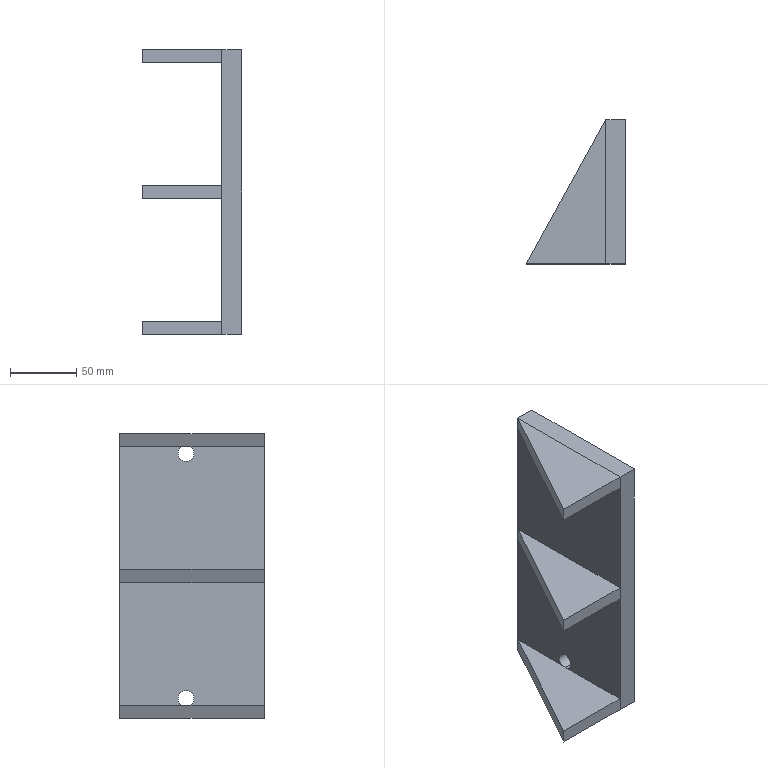Part | SolidWorks | features Extrusion 1, HoleWzd 1, ICE 1, LPattern 1, WeldmentFeature 1 | 4 solids | 30 faces | box 75 x 109 x 215 mm | volume 446232 mm3 | plane 23 | cylinder 7 | commonest cylinder face diameters 12 x7
STEP:
#1=CARTESIAN_POINT('',(-15.,0.,112.5));
#2=VERTEX_POINT('',#1);
#3=CARTESIAN_POINT('',(-15.,109.,112.5));
#4=VERTEX_POINT('',#3);
#5=CARTESIAN_POINT('',(-15.,0.,112.5));
#6=DIRECTION('',(0.,1.,0.));
#7=VECTOR('',#6,1000.);
#8=LINE('',#5,#7);
#9=EDGE_CURVE('',#2,#4,#8,.T.);
#10=ORIENTED_EDGE('',*,*,#9,.F.);
#11=CARTESIAN_POINT('',(-15.,0.,102.5));
#12=VERTEX_POINT('',#11);
#13=CARTESIAN_POINT('',(-15.,0.,102.5));
#14=DIRECTION('',(0.,0.,1.));
#15=VECTOR('',#14,1000.);
#16=LINE('',#13,#15);
#17=EDGE_CURVE('',#12,#2,#16,.T.);
#18=ORIENTED_EDGE('',*,*,#17,.F.);
#19=CARTESIAN_POINT('',(-15.,109.,102.5));
#20=VERTEX_POINT('',#19);
#21=CARTESIAN_POINT('',(-15.,0.,102.5));
#22=DIRECTION('',(0.,1.,0.));
#23=VECTOR('',#22,1000.);
#24=LINE('',#21,#23);
#25=EDGE_CURVE('',#12,#20,#24,.T.);
#26=ORIENTED_EDGE('',*,*,#25,.T.);
#27=CARTESIAN_POINT('',(-15.,109.,102.5));
#28=DIRECTION('',(0.,0.,1.));
#29=VECTOR('',#28,1000.);
#30=LINE('',#27,#29);
#31=EDGE_CURVE('',#20,#4,#30,.T.);
#32=ORIENTED_EDGE('',*,*,#31,.T.);
#33=EDGE_LOOP('',(#10,#18,#26,#32));
#34=FACE_OUTER_BOUND('',#33,.T.);
#35=CARTESIAN_POINT('',(-15.,0.,102.5));
#36=DIRECTION('',(1.,0.,0.));
#37=DIRECTION('',(0.,1.,0.));
#38=AXIS2_PLACEMENT_3D('',#35,#36,#37);
#39=PLANE('',#38);
#40=ADVANCED_FACE('',(#34),#39,.T.);
#41=CARTESIAN_POINT('',(-75.,0.,112.5));
#42=VERTEX_POINT('',#41);
#43=CARTESIAN_POINT('',(-75.,0.,112.5));
#44=DIRECTION('',(1.,0.,0.));
#45=VECTOR('',#44,1000.);
#46=LINE('',#43,#45);
#47=EDGE_CURVE('',#42,#2,#46,.T.);
#48=ORIENTED_EDGE('',*,*,#47,.F.);
#49=CARTESIAN_POINT('',(-75.,0.,102.5));
#50=VERTEX_POINT('',#49);
#51=CARTESIAN_POINT('',(-75.,0.,102.5));
#52=DIRECTION('',(0.,0.,1.));
#53=VECTOR('',#52,1000.);
#54=LINE('',#51,#53);
#55=EDGE_CURVE('',#50,#42,#54,.T.);
#56=ORIENTED_EDGE('',*,*,#55,.F.);
#57=CARTESIAN_POINT('',(-75.,0.,102.5));
#58=DIRECTION('',(1.,0.,0.));
#59=VECTOR('',#58,1000.);
#60=LINE('',#57,#59);
#61=EDGE_CURVE('',#50,#12,#60,.T.);
#62=ORIENTED_EDGE('',*,*,#61,.T.);
#63=ORIENTED_EDGE('',*,*,#17,.T.);
#64=EDGE_LOOP('',(#48,#56,#62,#63));
#65=FACE_OUTER_BOUND('',#64,.T.);
#66=CARTESIAN_POINT('',(-75.,0.,102.5));
#67=DIRECTION('',(0.,-1.,0.));
#68=DIRECTION('',(1.,0.,0.));
#69=AXIS2_PLACEMENT_3D('',#66,#67,#68);
#70=PLANE('',#69);
#71=ADVANCED_FACE('',(#65),#70,.T.);
#72=CARTESIAN_POINT('',(-15.,109.,112.5));
#73=DIRECTION('',(-0.4822,-0.876,0.));
#74=VECTOR('',#73,1000.);
#75=LINE('',#72,#74);
#76=EDGE_CURVE('',#4,#42,#75,.T.);
#77=ORIENTED_EDGE('',*,*,#76,.F.);
#78=ORIENTED_EDGE('',*,*,#31,.F.);
#79=CARTESIAN_POINT('',(-15.,109.,102.5));
#80=DIRECTION('',(-0.4822,-0.876,0.));
#81=VECTOR('',#80,1000.);
#82=LINE('',#79,#81);
#83=EDGE_CURVE('',#20,#50,#82,.T.);
#84=ORIENTED_EDGE('',*,*,#83,.T.);
#85=ORIENTED_EDGE('',*,*,#55,.T.);
#86=EDGE_LOOP('',(#77,#78,#84,#85));
#87=FACE_OUTER_BOUND('',#86,.T.);
#88=CARTESIAN_POINT('',(-15.,109.,102.5));
#89=DIRECTION('',(-0.876,0.4822,0.));
#90=DIRECTION('',(-0.4822,-0.876,0.));
#91=AXIS2_PLACEMENT_3D('',#88,#89,#90);
#92=PLANE('',#91);
#93=ADVANCED_FACE('',(#87),#92,.T.);
#94=ORIENTED_EDGE('',*,*,#25,.F.);
#95=ORIENTED_EDGE('',*,*,#61,.F.);
#96=ORIENTED_EDGE('',*,*,#83,.F.);
#97=EDGE_LOOP('',(#94,#95,#96));
#98=FACE_OUTER_BOUND('',#97,.T.);
#99=CARTESIAN_POINT('',(0.,0.,102.5));
#100=DIRECTION('',(0.,0.,-1.));
#101=DIRECTION('',(-1.,0.,0.));
#102=AXIS2_PLACEMENT_3D('',#99,#100,#101);
#103=PLANE('',#102);
#104=ADVANCED_FACE('',(#98),#103,.T.);
#105=ORIENTED_EDGE('',*,*,#9,.T.);
#106=ORIENTED_EDGE('',*,*,#76,.T.);
#107=ORIENTED_EDGE('',*,*,#47,.T.);
#108=EDGE_LOOP('',(#105,#106,#107));
#109=FACE_OUTER_BOUND('',#108,.T.);
#110=CARTESIAN_POINT('',(0.,0.,112.5));
#111=DIRECTION('',(0.,0.,-1.));
#112=DIRECTION('',(-1.,0.,0.));
#113=AXIS2_PLACEMENT_3D('',#110,#111,#112);
#114=PLANE('',#113);
#115=ADVANCED_FACE('',(#109),#114,.F.);
#116=CLOSED_SHELL('',(#40,#71,#93,#104,#115));
#117=MANIFOLD_SOLID_BREP('',#116);
#118=CARTESIAN_POINT('',(-15.,59.,206.));
#119=VERTEX_POINT('',#118);
#120=CARTESIAN_POINT('',(-15.,59.,194.));
#121=VERTEX_POINT('',#120);
#122=CARTESIAN_POINT('',(-15.,59.,200.));
#123=DIRECTION('',(1.,0.,0.));
#124=DIRECTION('',(0.,1.,0.));
#125=AXIS2_PLACEMENT_3D('',#122,#123,#124);
#126=CIRCLE('',#125,6.);
#127=EDGE_CURVE('',#119,#121,#126,.T.);
#128=ORIENTED_EDGE('',*,*,#127,.F.);
#129=CARTESIAN_POINT('',(0.,59.,206.));
#130=VERTEX_POINT('',#129);
#131=CARTESIAN_POINT('',(0.,59.,206.));
#132=DIRECTION('',(1.,0.,0.));
#133=VECTOR('',#132,1000.);
#134=LINE('',#131,#133);
#135=EDGE_CURVE('',#119,#130,#134,.T.);
#136=ORIENTED_EDGE('',*,*,#135,.T.);
#137=CARTESIAN_POINT('',(0.,59.,194.));
#138=VERTEX_POINT('',#137);
#139=CARTESIAN_POINT('',(0.,59.,200.));
#140=DIRECTION('',(1.,0.,0.));
#141=DIRECTION('',(0.,0.,-1.));
#142=AXIS2_PLACEMENT_3D('',#139,#140,#141);
#143=CIRCLE('',#142,6.);
#144=EDGE_CURVE('',#130,#138,#143,.T.);
#145=ORIENTED_EDGE('',*,*,#144,.T.);
#146=CARTESIAN_POINT('',(0.,59.,194.));
#147=DIRECTION('',(1.,0.,0.));
#148=VECTOR('',#147,1000.);
#149=LINE('',#146,#148);
#150=EDGE_CURVE('',#121,#138,#149,.T.);
#151=ORIENTED_EDGE('',*,*,#150,.F.);
#152=EDGE_LOOP('',(#128,#136,#145,#151));
#153=FACE_OUTER_BOUND('',#152,.T.);
#154=CARTESIAN_POINT('',(0.,59.,200.));
#155=DIRECTION('',(1.,0.,0.));
#156=DIRECTION('',(0.,0.,-1.));
#157=AXIS2_PLACEMENT_3D('',#154,#155,#156);
#158=CYLINDRICAL_SURFACE('',#157,6.);
#159=ADVANCED_FACE('',(#153),#158,.F.);
#160=CARTESIAN_POINT('',(-15.,59.,21.));
#161=VERTEX_POINT('',#160);
#162=CARTESIAN_POINT('',(-15.,59.,9.));
#163=VERTEX_POINT('',#162);
#164=CARTESIAN_POINT('',(-15.,59.,15.));
#165=DIRECTION('',(1.,0.,0.));
#166=DIRECTION('',(0.,1.,0.));
#167=AXIS2_PLACEMENT_3D('',#164,#165,#166);
#168=CIRCLE('',#167,6.);
#169=EDGE_CURVE('',#161,#163,#168,.T.);
#170=ORIENTED_EDGE('',*,*,#169,.F.);
#171=CARTESIAN_POINT('',(0.,59.,21.));
#172=VERTEX_POINT('',#171);
#173=CARTESIAN_POINT('',(0.,59.,21.));
#174=DIRECTION('',(1.,0.,0.));
#175=VECTOR('',#174,1000.);
#176=LINE('',#173,#175);
#177=EDGE_CURVE('',#161,#172,#176,.T.);
#178=ORIENTED_EDGE('',*,*,#177,.T.);
#179=CARTESIAN_POINT('',(0.,59.,9.));
#180=VERTEX_POINT('',#179);
#181=CARTESIAN_POINT('',(0.,59.,15.));
#182=DIRECTION('',(1.,0.,0.));
#183=DIRECTION('',(0.,0.,-1.));
#184=AXIS2_PLACEMENT_3D('',#181,#182,#183);
#185=CIRCLE('',#184,6.);
#186=EDGE_CURVE('',#172,#180,#185,.T.);
#187=ORIENTED_EDGE('',*,*,#186,.T.);
#188=CARTESIAN_POINT('',(0.,59.,9.));
#189=DIRECTION('',(1.,0.,0.));
#190=VECTOR('',#189,1000.);
#191=LINE('',#188,#190);
#192=EDGE_CURVE('',#163,#180,#191,.T.);
#193=ORIENTED_EDGE('',*,*,#192,.F.);
#194=EDGE_LOOP('',(#170,#178,#187,#193));
#195=FACE_OUTER_BOUND('',#194,.T.);
#196=CARTESIAN_POINT('',(0.,59.,15.));
#197=DIRECTION('',(1.,0.,0.));
#198=DIRECTION('',(0.,0.,-1.));
#199=AXIS2_PLACEMENT_3D('',#196,#197,#198);
#200=CYLINDRICAL_SURFACE('',#199,6.);
#201=ADVANCED_FACE('',(#195),#200,.F.);
#202=CARTESIAN_POINT('',(0.,0.,0.));
#203=VERTEX_POINT('',#202);
#204=CARTESIAN_POINT('',(0.,109.,0.));
#205=VERTEX_POINT('',#204);
#206=CARTESIAN_POINT('',(0.,109.,0.));
#207=DIRECTION('',(0.,1.,0.));
#208=VECTOR('',#207,1000.);
#209=LINE('',#206,#208);
#210=EDGE_CURVE('',#203,#205,#209,.T.);
#211=ORIENTED_EDGE('',*,*,#210,.T.);
#212=CARTESIAN_POINT('',(0.,109.,215.));
#213=VERTEX_POINT('',#212);
#214=CARTESIAN_POINT('',(0.,109.,215.));
#215=DIRECTION('',(0.,0.,-1.));
#216=VECTOR('',#215,1000.);
#217=LINE('',#214,#216);
#218=EDGE_CURVE('',#213,#205,#217,.T.);
#219=ORIENTED_EDGE('',*,*,#218,.F.);
#220=CARTESIAN_POINT('',(0.,0.,215.));
#221=VERTEX_POINT('',#220);
#222=CARTESIAN_POINT('',(0.,109.,215.));
#223=DIRECTION('',(0.,1.,0.));
#224=VECTOR('',#223,1000.);
#225=LINE('',#222,#224);
#226=EDGE_CURVE('',#221,#213,#225,.T.);
#227=ORIENTED_EDGE('',*,*,#226,.F.);
#228=CARTESIAN_POINT('',(0.,0.,215.));
#229=DIRECTION('',(0.,0.,-1.));
#230=VECTOR('',#229,1000.);
#231=LINE('',#228,#230);
#232=EDGE_CURVE('',#221,#203,#231,.T.);
#233=ORIENTED_EDGE('',*,*,#232,.T.);
#234=EDGE_LOOP('',(#211,#219,#227,#233));
#235=FACE_OUTER_BOUND('',#234,.T.);
#236=CARTESIAN_POINT('',(0.,59.,15.));
#237=DIRECTION('',(1.,0.,0.));
#238=DIRECTION('',(0.,0.,-1.));
#239=AXIS2_PLACEMENT_3D('',#236,#237,#238);
#240=CIRCLE('',#239,6.);
#241=EDGE_CURVE('',#180,#172,#240,.T.);
#242=ORIENTED_EDGE('',*,*,#241,.F.);
#243=ORIENTED_EDGE('',*,*,#186,.F.);
#244=EDGE_LOOP('',(#242,#243));
#245=FACE_BOUND('',#244,.T.);
#246=CARTESIAN_POINT('',(0.,59.,200.));
#247=DIRECTION('',(1.,0.,0.));
#248=DIRECTION('',(0.,0.,-1.));
#249=AXIS2_PLACEMENT_3D('',#246,#247,#248);
#250=CIRCLE('',#249,6.);
#251=EDGE_CURVE('',#138,#130,#250,.T.);
#252=ORIENTED_EDGE('',*,*,#251,.F.);
#253=ORIENTED_EDGE('',*,*,#144,.F.);
#254=EDGE_LOOP('',(#252,#253));
#255=FACE_BOUND('',#254,.T.);
#256=CARTESIAN_POINT('',(0.,109.,215.));
#257=DIRECTION('',(-1.,0.,0.));
#258=DIRECTION('',(0.,-1.,0.));
#259=AXIS2_PLACEMENT_3D('',#256,#257,#258);
#260=PLANE('',#259);
#261=ADVANCED_FACE('',(#235,#245,#255),#260,.F.);
#262=CARTESIAN_POINT('',(-15.,109.,0.));
#263=VERTEX_POINT('',#262);
#264=CARTESIAN_POINT('',(-15.,109.,0.));
#265=DIRECTION('',(-1.,0.,0.));
#266=VECTOR('',#265,1000.);
#267=LINE('',#264,#266);
#268=EDGE_CURVE('',#205,#263,#267,.T.);
#269=ORIENTED_EDGE('',*,*,#268,.T.);
#270=CARTESIAN_POINT('',(-15.,109.,215.));
#271=VERTEX_POINT('',#270);
#272=CARTESIAN_POINT('',(-15.,109.,215.));
#273=DIRECTION('',(0.,0.,-1.));
#274=VECTOR('',#273,1000.);
#275=LINE('',#272,#274);
#276=EDGE_CURVE('',#271,#263,#275,.T.);
#277=ORIENTED_EDGE('',*,*,#276,.F.);
#278=CARTESIAN_POINT('',(-15.,109.,215.));
#279=DIRECTION('',(-1.,0.,0.));
#280=VECTOR('',#279,1000.);
#281=LINE('',#278,#280);
#282=EDGE_CURVE('',#213,#271,#281,.T.);
#283=ORIENTED_EDGE('',*,*,#282,.F.);
#284=ORIENTED_EDGE('',*,*,#218,.T.);
#285=EDGE_LOOP('',(#269,#277,#283,#284));
#286=FACE_OUTER_BOUND('',#285,.T.);
#287=CARTESIAN_POINT('',(-15.,109.,215.));
#288=DIRECTION('',(0.,-1.,0.));
#289=DIRECTION('',(0.,0.,-1.));
#290=AXIS2_PLACEMENT_3D('',#287,#288,#289);
#291=PLANE('',#290);
#292=ADVANCED_FACE('',(#286),#291,.F.);
#293=CARTESIAN_POINT('',(-15.,59.,200.));
#294=DIRECTION('',(1.,0.,0.));
#295=DIRECTION('',(0.,1.,0.));
#296=AXIS2_PLACEMENT_3D('',#293,#294,#295);
#297=CIRCLE('',#296,6.);
#298=EDGE_CURVE('',#121,#119,#297,.T.);
#299=ORIENTED_EDGE('',*,*,#298,.T.);
#300=ORIENTED_EDGE('',*,*,#127,.T.);
#301=EDGE_LOOP('',(#299,#300));
#302=FACE_BOUND('',#301,.T.);
#303=CARTESIAN_POINT('',(-15.,59.,15.));
#304=DIRECTION('',(1.,0.,0.));
#305=DIRECTION('',(0.,1.,0.));
#306=AXIS2_PLACEMENT_3D('',#303,#304,#305);
#307=CIRCLE('',#306,6.);
#308=EDGE_CURVE('',#163,#161,#307,.T.);
#309=ORIENTED_EDGE('',*,*,#308,.T.);
#310=ORIENTED_EDGE('',*,*,#169,.T.);
#311=EDGE_LOOP('',(#309,#310));
#312=FACE_BOUND('',#311,.T.);
#313=CARTESIAN_POINT('',(-15.,0.,0.));
#314=VERTEX_POINT('',#313);
#315=CARTESIAN_POINT('',(-15.,109.,0.));
#316=DIRECTION('',(0.,-1.,0.));
#317=VECTOR('',#316,1000.);
#318=LINE('',#315,#317);
#319=EDGE_CURVE('',#263,#314,#318,.T.);
#320=ORIENTED_EDGE('',*,*,#319,.T.);
#321=CARTESIAN_POINT('',(-15.,0.,215.));
#322=VERTEX_POINT('',#321);
#323=CARTESIAN_POINT('',(-15.,0.,215.));
#324=DIRECTION('',(0.,0.,-1.));
#325=VECTOR('',#324,1000.);
#326=LINE('',#323,#325);
#327=EDGE_CURVE('',#322,#314,#326,.T.);
#328=ORIENTED_EDGE('',*,*,#327,.F.);
#329=CARTESIAN_POINT('',(-15.,109.,215.));
#330=DIRECTION('',(0.,-1.,0.));
#331=VECTOR('',#330,1000.);
#332=LINE('',#329,#331);
#333=EDGE_CURVE('',#271,#322,#332,.T.);
#334=ORIENTED_EDGE('',*,*,#333,.F.);
#335=ORIENTED_EDGE('',*,*,#276,.T.);
#336=EDGE_LOOP('',(#320,#328,#334,#335));
#337=FACE_OUTER_BOUND('',#336,.T.);
#338=CARTESIAN_POINT('',(-15.,109.,215.));
#339=DIRECTION('',(1.,0.,0.));
#340=DIRECTION('',(0.,1.,0.));
#341=AXIS2_PLACEMENT_3D('',#338,#339,#340);
#342=PLANE('',#341);
#343=ADVANCED_FACE('',(#302,#312,#337),#342,.F.);
#344=CARTESIAN_POINT('',(0.,0.,0.));
#345=DIRECTION('',(1.,0.,0.));
#346=VECTOR('',#345,1000.);
#347=LINE('',#344,#346);
#348=EDGE_CURVE('',#314,#203,#347,.T.);
#349=ORIENTED_EDGE('',*,*,#348,.T.);
#350=ORIENTED_EDGE('',*,*,#232,.F.);
#351=CARTESIAN_POINT('',(0.,0.,215.));
#352=DIRECTION('',(1.,0.,0.));
#353=VECTOR('',#352,1000.);
#354=LINE('',#351,#353);
#355=EDGE_CURVE('',#322,#221,#354,.T.);
#356=ORIENTED_EDGE('',*,*,#355,.F.);
#357=ORIENTED_EDGE('',*,*,#327,.T.);
#358=EDGE_LOOP('',(#349,#350,#356,#357));
#359=FACE_OUTER_BOUND('',#358,.T.);
#360=CARTESIAN_POINT('',(0.,0.,215.));
#361=DIRECTION('',(0.,1.,0.));
#362=DIRECTION('',(-1.,0.,0.));
#363=AXIS2_PLACEMENT_3D('',#360,#361,#362);
#364=PLANE('',#363);
#365=ADVANCED_FACE('',(#359),#364,.F.);
#366=ORIENTED_EDGE('',*,*,#282,.T.);
#367=ORIENTED_EDGE('',*,*,#333,.T.);
#368=ORIENTED_EDGE('',*,*,#355,.T.);
#369=ORIENTED_EDGE('',*,*,#226,.T.);
#370=EDGE_LOOP('',(#366,#367,#368,#369));
#371=FACE_OUTER_BOUND('',#370,.T.);
#372=CARTESIAN_POINT('',(0.,0.,215.));
#373=DIRECTION('',(0.,0.,-1.));
#374=DIRECTION('',(-1.,0.,0.));
#375=AXIS2_PLACEMENT_3D('',#372,#373,#374);
#376=PLANE('',#375);
#377=ADVANCED_FACE('',(#371),#376,.F.);
#378=ORIENTED_EDGE('',*,*,#268,.F.);
#379=ORIENTED_EDGE('',*,*,#210,.F.);
#380=ORIENTED_EDGE('',*,*,#348,.F.);
#381=ORIENTED_EDGE('',*,*,#319,.F.);
#382=EDGE_LOOP('',(#378,#379,#380,#381));
#383=FACE_OUTER_BOUND('',#382,.T.);
#384=CARTESIAN_POINT('',(0.,0.,0.));
#385=DIRECTION('',(0.,0.,-1.));
#386=DIRECTION('',(-1.,0.,0.));
#387=AXIS2_PLACEMENT_3D('',#384,#385,#386);
#388=PLANE('',#387);
#389=ADVANCED_FACE('',(#383),#388,.T.);
#390=ORIENTED_EDGE('',*,*,#177,.F.);
#391=ORIENTED_EDGE('',*,*,#308,.F.);
#392=ORIENTED_EDGE('',*,*,#192,.T.);
#393=ORIENTED_EDGE('',*,*,#241,.T.);
#394=EDGE_LOOP('',(#390,#391,#392,#393));
#395=FACE_OUTER_BOUND('',#394,.T.);
#396=CARTESIAN_POINT('',(0.,59.,15.));
#397=DIRECTION('',(1.,0.,0.));
#398=DIRECTION('',(0.,0.,-1.));
#399=AXIS2_PLACEMENT_3D('',#396,#397,#398);
#400=CYLINDRICAL_SURFACE('',#399,6.);
#401=ADVANCED_FACE('',(#395),#400,.F.);
#402=ORIENTED_EDGE('',*,*,#135,.F.);
#403=ORIENTED_EDGE('',*,*,#298,.F.);
#404=ORIENTED_EDGE('',*,*,#150,.T.);
#405=ORIENTED_EDGE('',*,*,#251,.T.);
#406=EDGE_LOOP('',(#402,#403,#404,#405));
#407=FACE_OUTER_BOUND('',#406,.T.);
#408=CARTESIAN_POINT('',(0.,59.,200.));
#409=DIRECTION('',(1.,0.,0.));
#410=DIRECTION('',(0.,0.,-1.));
#411=AXIS2_PLACEMENT_3D('',#408,#409,#410);
#412=CYLINDRICAL_SURFACE('',#411,6.);
#413=ADVANCED_FACE('',(#407),#412,.F.);
#414=CLOSED_SHELL('',(#159,#201,#261,#292,#343,#365,#377,#389,#401,#413));
#415=MANIFOLD_SOLID_BREP('',#414);
#416=CARTESIAN_POINT('',(-15.,62.317,205.));
#417=VERTEX_POINT('',#416);
#418=CARTESIAN_POINT('',(-15.,55.683,205.));
#419=VERTEX_POINT('',#418);
#420=CARTESIAN_POINT('',(-15.,59.,200.));
#421=DIRECTION('',(1.,0.,0.));
#422=DIRECTION('',(0.,1.,0.));
#423=AXIS2_PLACEMENT_3D('',#420,#421,#422);
#424=CIRCLE('',#423,6.);
#425=EDGE_CURVE('',#417,#419,#424,.T.);
#426=ORIENTED_EDGE('',*,*,#425,.F.);
#427=CARTESIAN_POINT('',(-15.,109.,205.));
#428=VERTEX_POINT('',#427);
#429=CARTESIAN_POINT('',(-15.,0.,205.));
#430=DIRECTION('',(0.,1.,0.));
#431=VECTOR('',#430,1000.);
#432=LINE('',#429,#431);
#433=EDGE_CURVE('',#417,#428,#432,.T.);
#434=ORIENTED_EDGE('',*,*,#433,.T.);
#435=CARTESIAN_POINT('',(-15.,109.,215.));
#436=VERTEX_POINT('',#435);
#437=CARTESIAN_POINT('',(-15.,109.,205.));
#438=DIRECTION('',(0.,0.,1.));
#439=VECTOR('',#438,1000.);
#440=LINE('',#437,#439);
#441=EDGE_CURVE('',#428,#436,#440,.T.);
#442=ORIENTED_EDGE('',*,*,#441,.T.);
#443=CARTESIAN_POINT('',(-15.,0.,215.));
#444=VERTEX_POINT('',#443);
#445=CARTESIAN_POINT('',(-15.,0.,215.));
#446=DIRECTION('',(0.,1.,0.));
#447=VECTOR('',#446,1000.);
#448=LINE('',#445,#447);
#449=EDGE_CURVE('',#444,#436,#448,.T.);
#450=ORIENTED_EDGE('',*,*,#449,.F.);
#451=CARTESIAN_POINT('',(-15.,0.,205.));
#452=VERTEX_POINT('',#451);
#453=CARTESIAN_POINT('',(-15.,0.,205.));
#454=DIRECTION('',(0.,0.,1.));
#455=VECTOR('',#454,1000.);
#456=LINE('',#453,#455);
#457=EDGE_CURVE('',#452,#444,#456,.T.);
#458=ORIENTED_EDGE('',*,*,#457,.F.);
#459=CARTESIAN_POINT('',(-15.,0.,205.));
#460=DIRECTION('',(0.,1.,0.));
#461=VECTOR('',#460,1000.);
#462=LINE('',#459,#461);
#463=EDGE_CURVE('',#452,#419,#462,.T.);
#464=ORIENTED_EDGE('',*,*,#463,.T.);
#465=EDGE_LOOP('',(#426,#434,#442,#450,#458,#464));
#466=FACE_OUTER_BOUND('',#465,.T.);
#467=CARTESIAN_POINT('',(-15.,0.,205.));
#468=DIRECTION('',(1.,0.,0.));
#469=DIRECTION('',(0.,1.,0.));
#470=AXIS2_PLACEMENT_3D('',#467,#468,#469);
#471=PLANE('',#470);
#472=ADVANCED_FACE('',(#466),#471,.T.);
#473=CARTESIAN_POINT('',(-75.,0.,215.));
#474=VERTEX_POINT('',#473);
#475=CARTESIAN_POINT('',(-75.,0.,215.));
#476=DIRECTION('',(1.,0.,0.));
#477=VECTOR('',#476,1000.);
#478=LINE('',#475,#477);
#479=EDGE_CURVE('',#474,#444,#478,.T.);
#480=ORIENTED_EDGE('',*,*,#479,.F.);
#481=CARTESIAN_POINT('',(-75.,0.,205.));
#482=VERTEX_POINT('',#481);
#483=CARTESIAN_POINT('',(-75.,0.,205.));
#484=DIRECTION('',(0.,0.,1.));
#485=VECTOR('',#484,1000.);
#486=LINE('',#483,#485);
#487=EDGE_CURVE('',#482,#474,#486,.T.);
#488=ORIENTED_EDGE('',*,*,#487,.F.);
#489=CARTESIAN_POINT('',(-75.,0.,205.));
#490=DIRECTION('',(1.,0.,0.));
#491=VECTOR('',#490,1000.);
#492=LINE('',#489,#491);
#493=EDGE_CURVE('',#482,#452,#492,.T.);
#494=ORIENTED_EDGE('',*,*,#493,.T.);
#495=ORIENTED_EDGE('',*,*,#457,.T.);
#496=EDGE_LOOP('',(#480,#488,#494,#495));
#497=FACE_OUTER_BOUND('',#496,.T.);
#498=CARTESIAN_POINT('',(-75.,0.,205.));
#499=DIRECTION('',(0.,-1.,0.));
#500=DIRECTION('',(1.,0.,0.));
#501=AXIS2_PLACEMENT_3D('',#498,#499,#500);
#502=PLANE('',#501);
#503=ADVANCED_FACE('',(#497),#502,.T.);
#504=CARTESIAN_POINT('',(-15.,109.,215.));
#505=DIRECTION('',(-0.4822,-0.876,0.));
#506=VECTOR('',#505,1000.);
#507=LINE('',#504,#506);
#508=EDGE_CURVE('',#436,#474,#507,.T.);
#509=ORIENTED_EDGE('',*,*,#508,.F.);
#510=ORIENTED_EDGE('',*,*,#441,.F.);
#511=CARTESIAN_POINT('',(-15.,109.,205.));
#512=DIRECTION('',(-0.4822,-0.876,0.));
#513=VECTOR('',#512,1000.);
#514=LINE('',#511,#513);
#515=EDGE_CURVE('',#428,#482,#514,.T.);
#516=ORIENTED_EDGE('',*,*,#515,.T.);
#517=ORIENTED_EDGE('',*,*,#487,.T.);
#518=EDGE_LOOP('',(#509,#510,#516,#517));
#519=FACE_OUTER_BOUND('',#518,.T.);
#520=CARTESIAN_POINT('',(-15.,109.,205.));
#521=DIRECTION('',(-0.876,0.4822,0.));
#522=DIRECTION('',(-0.4822,-0.876,0.));
#523=AXIS2_PLACEMENT_3D('',#520,#521,#522);
#524=PLANE('',#523);
#525=ADVANCED_FACE('',(#519),#524,.T.);
#526=CARTESIAN_POINT('',(-15.001,62.317,205.));
#527=VERTEX_POINT('',#526);
#528=CARTESIAN_POINT('',(0.,62.317,205.));
#529=DIRECTION('',(1.,0.,0.));
#530=VECTOR('',#529,1000.);
#531=LINE('',#528,#530);
#532=EDGE_CURVE('',#527,#417,#531,.T.);
#533=ORIENTED_EDGE('',*,*,#532,.F.);
#534=CARTESIAN_POINT('',(-15.001,55.683,205.));
#535=VERTEX_POINT('',#534);
#536=CARTESIAN_POINT('',(-15.001,0.,205.));
#537=DIRECTION('',(0.,1.,0.));
#538=VECTOR('',#537,1000.);
#539=LINE('',#536,#538);
#540=EDGE_CURVE('',#535,#527,#539,.T.);
#541=ORIENTED_EDGE('',*,*,#540,.F.);
#542=CARTESIAN_POINT('',(0.,55.683,205.));
#543=DIRECTION('',(-1.,0.,0.));
#544=VECTOR('',#543,1000.);
#545=LINE('',#542,#544);
#546=EDGE_CURVE('',#419,#535,#545,.T.);
#547=ORIENTED_EDGE('',*,*,#546,.F.);
#548=ORIENTED_EDGE('',*,*,#463,.F.);
#549=ORIENTED_EDGE('',*,*,#493,.F.);
#550=ORIENTED_EDGE('',*,*,#515,.F.);
#551=ORIENTED_EDGE('',*,*,#433,.F.);
#552=EDGE_LOOP('',(#533,#541,#547,#548,#549,#550,#551));
#553=FACE_OUTER_BOUND('',#552,.T.);
#554=CARTESIAN_POINT('',(0.,0.,205.));
#555=DIRECTION('',(0.,0.,-1.));
#556=DIRECTION('',(-1.,0.,0.));
#557=AXIS2_PLACEMENT_3D('',#554,#555,#556);
#558=PLANE('',#557);
#559=ADVANCED_FACE('',(#553),#558,.T.);
#560=ORIENTED_EDGE('',*,*,#449,.T.);
#561=ORIENTED_EDGE('',*,*,#508,.T.);
#562=ORIENTED_EDGE('',*,*,#479,.T.);
#563=EDGE_LOOP('',(#560,#561,#562));
#564=FACE_OUTER_BOUND('',#563,.T.);
#565=CARTESIAN_POINT('',(0.,0.,215.));
#566=DIRECTION('',(0.,0.,-1.));
#567=DIRECTION('',(-1.,0.,0.));
#568=AXIS2_PLACEMENT_3D('',#565,#566,#567);
#569=PLANE('',#568);
#570=ADVANCED_FACE('',(#564),#569,.F.);
#571=ORIENTED_EDGE('',*,*,#540,.T.);
#572=CARTESIAN_POINT('',(-15.001,59.,200.));
#573=DIRECTION('',(1.,0.,0.));
#574=DIRECTION('',(0.,0.,-1.));
#575=AXIS2_PLACEMENT_3D('',#572,#573,#574);
#576=CIRCLE('',#575,6.);
#577=EDGE_CURVE('',#527,#535,#576,.T.);
#578=ORIENTED_EDGE('',*,*,#577,.T.);
#579=EDGE_LOOP('',(#571,#578));
#580=FACE_OUTER_BOUND('',#579,.T.);
#581=CARTESIAN_POINT('',(-15.001,59.,200.));
#582=DIRECTION('',(-1.,0.,0.));
#583=DIRECTION('',(0.,0.,1.));
#584=AXIS2_PLACEMENT_3D('',#581,#582,#583);
#585=PLANE('',#584);
#586=ADVANCED_FACE('',(#580),#585,.F.);
#587=ORIENTED_EDGE('',*,*,#532,.T.);
#588=ORIENTED_EDGE('',*,*,#425,.T.);
#589=ORIENTED_EDGE('',*,*,#546,.T.);
#590=ORIENTED_EDGE('',*,*,#577,.F.);
#591=EDGE_LOOP('',(#587,#588,#589,#590));
#592=FACE_OUTER_BOUND('',#591,.T.);
#593=CARTESIAN_POINT('',(0.,59.,200.));
#594=DIRECTION('',(1.,0.,0.));
#595=DIRECTION('',(0.,0.,-1.));
#596=AXIS2_PLACEMENT_3D('',#593,#594,#595);
#597=CYLINDRICAL_SURFACE('',#596,6.);
#598=ADVANCED_FACE('',(#592),#597,.F.);
#599=CLOSED_SHELL('',(#472,#503,#525,#559,#570,#586,#598));
#600=MANIFOLD_SOLID_BREP('',#599);
#601=CARTESIAN_POINT('',(-15.001,59.,9.));
#602=VERTEX_POINT('',#601);
#603=CARTESIAN_POINT('',(-15.001,62.317,10.));
#604=VERTEX_POINT('',#603);
#605=CARTESIAN_POINT('',(-15.001,59.,15.));
#606=DIRECTION('',(1.,0.,0.));
#607=DIRECTION('',(0.,0.,-1.));
#608=AXIS2_PLACEMENT_3D('',#605,#606,#607);
#609=CIRCLE('',#608,6.);
#610=EDGE_CURVE('',#602,#604,#609,.T.);
#611=ORIENTED_EDGE('',*,*,#610,.F.);
#612=CARTESIAN_POINT('',(-15.,59.,9.));
#613=VERTEX_POINT('',#612);
#614=CARTESIAN_POINT('',(0.,59.,9.));
#615=DIRECTION('',(1.,0.,0.));
#616=VECTOR('',#615,1000.);
#617=LINE('',#614,#616);
#618=EDGE_CURVE('',#602,#613,#617,.T.);
#619=ORIENTED_EDGE('',*,*,#618,.T.);
#620=CARTESIAN_POINT('',(-15.,62.317,10.));
#621=VERTEX_POINT('',#620);
#622=CARTESIAN_POINT('',(-15.,59.,15.));
#623=DIRECTION('',(1.,0.,0.));
#624=DIRECTION('',(0.,1.,0.));
#625=AXIS2_PLACEMENT_3D('',#622,#623,#624);
#626=CIRCLE('',#625,6.);
#627=EDGE_CURVE('',#613,#621,#626,.T.);
#628=ORIENTED_EDGE('',*,*,#627,.T.);
#629=CARTESIAN_POINT('',(0.,62.317,10.));
#630=DIRECTION('',(1.,0.,0.));
#631=VECTOR('',#630,1000.);
#632=LINE('',#629,#631);
#633=EDGE_CURVE('',#604,#621,#632,.T.);
#634=ORIENTED_EDGE('',*,*,#633,.F.);
#635=EDGE_LOOP('',(#611,#619,#628,#634));
#636=FACE_OUTER_BOUND('',#635,.T.);
#637=CARTESIAN_POINT('',(0.,59.,15.));
#638=DIRECTION('',(1.,0.,0.));
#639=DIRECTION('',(0.,0.,-1.));
#640=AXIS2_PLACEMENT_3D('',#637,#638,#639);
#641=CYLINDRICAL_SURFACE('',#640,6.);
#642=ADVANCED_FACE('',(#636),#641,.F.);
#643=CARTESIAN_POINT('',(-15.,55.683,10.));
#644=VERTEX_POINT('',#643);
#645=CARTESIAN_POINT('',(-15.,59.,15.));
#646=DIRECTION('',(1.,0.,0.));
#647=DIRECTION('',(0.,1.,0.));
#648=AXIS2_PLACEMENT_3D('',#645,#646,#647);
#649=CIRCLE('',#648,6.);
#650=EDGE_CURVE('',#644,#613,#649,.T.);
#651=ORIENTED_EDGE('',*,*,#650,.F.);
#652=CARTESIAN_POINT('',(-15.,0.,10.));
#653=VERTEX_POINT('',#652);
#654=CARTESIAN_POINT('',(-15.,0.,10.));
#655=DIRECTION('',(0.,1.,0.));
#656=VECTOR('',#655,1000.);
#657=LINE('',#654,#656);
#658=EDGE_CURVE('',#653,#644,#657,.T.);
#659=ORIENTED_EDGE('',*,*,#658,.F.);
#660=CARTESIAN_POINT('',(-15.,0.,0.));
#661=VERTEX_POINT('',#660);
#662=CARTESIAN_POINT('',(-15.,0.,0.));
#663=DIRECTION('',(0.,0.,1.));
#664=VECTOR('',#663,1000.);
#665=LINE('',#662,#664);
#666=EDGE_CURVE('',#661,#653,#665,.T.);
#667=ORIENTED_EDGE('',*,*,#666,.F.);
#668=CARTESIAN_POINT('',(-15.,109.,0.));
#669=VERTEX_POINT('',#668);
#670=CARTESIAN_POINT('',(-15.,0.,0.));
#671=DIRECTION('',(0.,1.,0.));
#672=VECTOR('',#671,1000.);
#673=LINE('',#670,#672);
#674=EDGE_CURVE('',#661,#669,#673,.T.);
#675=ORIENTED_EDGE('',*,*,#674,.T.);
#676=CARTESIAN_POINT('',(-15.,109.,10.));
#677=VERTEX_POINT('',#676);
#678=CARTESIAN_POINT('',(-15.,109.,0.));
#679=DIRECTION('',(0.,0.,1.));
#680=VECTOR('',#679,1000.);
#681=LINE('',#678,#680);
#682=EDGE_CURVE('',#669,#677,#681,.T.);
#683=ORIENTED_EDGE('',*,*,#682,.T.);
#684=CARTESIAN_POINT('',(-15.,0.,10.));
#685=DIRECTION('',(0.,1.,0.));
#686=VECTOR('',#685,1000.);
#687=LINE('',#684,#686);
#688=EDGE_CURVE('',#621,#677,#687,.T.);
#689=ORIENTED_EDGE('',*,*,#688,.F.);
#690=ORIENTED_EDGE('',*,*,#627,.F.);
#691=EDGE_LOOP('',(#651,#659,#667,#675,#683,#689,#690));
#692=FACE_OUTER_BOUND('',#691,.T.);
#693=CARTESIAN_POINT('',(-15.,0.,0.));
#694=DIRECTION('',(1.,0.,0.));
#695=DIRECTION('',(0.,1.,0.));
#696=AXIS2_PLACEMENT_3D('',#693,#694,#695);
#697=PLANE('',#696);
#698=ADVANCED_FACE('',(#692),#697,.T.);
#699=CARTESIAN_POINT('',(-75.,0.,10.));
#700=VERTEX_POINT('',#699);
#701=CARTESIAN_POINT('',(-75.,0.,10.));
#702=DIRECTION('',(1.,0.,0.));
#703=VECTOR('',#702,1000.);
#704=LINE('',#701,#703);
#705=EDGE_CURVE('',#700,#653,#704,.T.);
#706=ORIENTED_EDGE('',*,*,#705,.F.);
#707=CARTESIAN_POINT('',(-75.,0.,0.));
#708=VERTEX_POINT('',#707);
#709=CARTESIAN_POINT('',(-75.,0.,0.));
#710=DIRECTION('',(0.,0.,1.));
#711=VECTOR('',#710,1000.);
#712=LINE('',#709,#711);
#713=EDGE_CURVE('',#708,#700,#712,.T.);
#714=ORIENTED_EDGE('',*,*,#713,.F.);
#715=CARTESIAN_POINT('',(-75.,0.,0.));
#716=DIRECTION('',(1.,0.,0.));
#717=VECTOR('',#716,1000.);
#718=LINE('',#715,#717);
#719=EDGE_CURVE('',#708,#661,#718,.T.);
#720=ORIENTED_EDGE('',*,*,#719,.T.);
#721=ORIENTED_EDGE('',*,*,#666,.T.);
#722=EDGE_LOOP('',(#706,#714,#720,#721));
#723=FACE_OUTER_BOUND('',#722,.T.);
#724=CARTESIAN_POINT('',(-75.,0.,0.));
#725=DIRECTION('',(0.,-1.,0.));
#726=DIRECTION('',(1.,0.,0.));
#727=AXIS2_PLACEMENT_3D('',#724,#725,#726);
#728=PLANE('',#727);
#729=ADVANCED_FACE('',(#723),#728,.T.);
#730=CARTESIAN_POINT('',(-15.,109.,10.));
#731=DIRECTION('',(-0.4822,-0.876,0.));
#732=VECTOR('',#731,1000.);
#733=LINE('',#730,#732);
#734=EDGE_CURVE('',#677,#700,#733,.T.);
#735=ORIENTED_EDGE('',*,*,#734,.F.);
#736=ORIENTED_EDGE('',*,*,#682,.F.);
#737=CARTESIAN_POINT('',(-15.,109.,0.));
#738=DIRECTION('',(-0.4822,-0.876,0.));
#739=VECTOR('',#738,1000.);
#740=LINE('',#737,#739);
#741=EDGE_CURVE('',#669,#708,#740,.T.);
#742=ORIENTED_EDGE('',*,*,#741,.T.);
#743=ORIENTED_EDGE('',*,*,#713,.T.);
#744=EDGE_LOOP('',(#735,#736,#742,#743));
#745=FACE_OUTER_BOUND('',#744,.T.);
#746=CARTESIAN_POINT('',(-15.,109.,0.));
#747=DIRECTION('',(-0.876,0.4822,0.));
#748=DIRECTION('',(-0.4822,-0.876,0.));
#749=AXIS2_PLACEMENT_3D('',#746,#747,#748);
#750=PLANE('',#749);
#751=ADVANCED_FACE('',(#745),#750,.T.);
#752=ORIENTED_EDGE('',*,*,#674,.F.);
#753=ORIENTED_EDGE('',*,*,#719,.F.);
#754=ORIENTED_EDGE('',*,*,#741,.F.);
#755=EDGE_LOOP('',(#752,#753,#754));
#756=FACE_OUTER_BOUND('',#755,.T.);
#757=CARTESIAN_POINT('',(0.,0.,0.));
#758=DIRECTION('',(0.,0.,-1.));
#759=DIRECTION('',(-1.,0.,0.));
#760=AXIS2_PLACEMENT_3D('',#757,#758,#759);
#761=PLANE('',#760);
#762=ADVANCED_FACE('',(#756),#761,.T.);
#763=CARTESIAN_POINT('',(-15.001,55.683,10.));
#764=VERTEX_POINT('',#763);
#765=CARTESIAN_POINT('',(-15.001,0.,10.));
#766=DIRECTION('',(0.,1.,0.));
#767=VECTOR('',#766,1000.);
#768=LINE('',#765,#767);
#769=EDGE_CURVE('',#764,#604,#768,.T.);
#770=ORIENTED_EDGE('',*,*,#769,.T.);
#771=ORIENTED_EDGE('',*,*,#633,.T.);
#772=ORIENTED_EDGE('',*,*,#688,.T.);
#773=ORIENTED_EDGE('',*,*,#734,.T.);
#774=ORIENTED_EDGE('',*,*,#705,.T.);
#775=ORIENTED_EDGE('',*,*,#658,.T.);
#776=CARTESIAN_POINT('',(0.,55.683,10.));
#777=DIRECTION('',(-1.,0.,0.));
#778=VECTOR('',#777,1000.);
#779=LINE('',#776,#778);
#780=EDGE_CURVE('',#644,#764,#779,.T.);
#781=ORIENTED_EDGE('',*,*,#780,.T.);
#782=EDGE_LOOP('',(#770,#771,#772,#773,#774,#775,#781));
#783=FACE_OUTER_BOUND('',#782,.T.);
#784=CARTESIAN_POINT('',(0.,0.,10.));
#785=DIRECTION('',(0.,0.,-1.));
#786=DIRECTION('',(-1.,0.,0.));
#787=AXIS2_PLACEMENT_3D('',#784,#785,#786);
#788=PLANE('',#787);
#789=ADVANCED_FACE('',(#783),#788,.F.);
#790=CARTESIAN_POINT('',(-15.001,59.,15.));
#791=DIRECTION('',(1.,0.,0.));
#792=DIRECTION('',(0.,0.,-1.));
#793=AXIS2_PLACEMENT_3D('',#790,#791,#792);
#794=CIRCLE('',#793,6.);
#795=EDGE_CURVE('',#764,#602,#794,.T.);
#796=ORIENTED_EDGE('',*,*,#795,.T.);
#797=ORIENTED_EDGE('',*,*,#610,.T.);
#798=ORIENTED_EDGE('',*,*,#769,.F.);
#799=EDGE_LOOP('',(#796,#797,#798));
#800=FACE_OUTER_BOUND('',#799,.T.);
#801=CARTESIAN_POINT('',(-15.001,59.,15.));
#802=DIRECTION('',(-1.,0.,0.));
#803=DIRECTION('',(0.,0.,1.));
#804=AXIS2_PLACEMENT_3D('',#801,#802,#803);
#805=PLANE('',#804);
#806=ADVANCED_FACE('',(#800),#805,.F.);
#807=ORIENTED_EDGE('',*,*,#618,.F.);
#808=ORIENTED_EDGE('',*,*,#795,.F.);
#809=ORIENTED_EDGE('',*,*,#780,.F.);
#810=ORIENTED_EDGE('',*,*,#650,.T.);
#811=EDGE_LOOP('',(#807,#808,#809,#810));
#812=FACE_OUTER_BOUND('',#811,.T.);
#813=CARTESIAN_POINT('',(0.,59.,15.));
#814=DIRECTION('',(1.,0.,0.));
#815=DIRECTION('',(0.,0.,-1.));
#816=AXIS2_PLACEMENT_3D('',#813,#814,#815);
#817=CYLINDRICAL_SURFACE('',#816,6.);
#818=ADVANCED_FACE('',(#812),#817,.F.);
#819=CLOSED_SHELL('',(#642,#698,#729,#751,#762,#789,#806,#818));
#820=MANIFOLD_SOLID_BREP('',#819);
#821=CARTESIAN_POINT('',(0.,0.,0.));
#822=DIRECTION('',(0.,0.,1.));
#823=DIRECTION('',(1.,0.,0.));
#824=AXIS2_PLACEMENT_3D('',#821,#822,#823);
#825=(LENGTH_UNIT()NAMED_UNIT(*)SI_UNIT(.MILLI.,.METRE.));
#826=UNCERTAINTY_MEASURE_WITH_UNIT(LENGTH_MEASURE(0.00001),#825,'','');
#827=(NAMED_UNIT(*)PLANE_ANGLE_UNIT()SI_UNIT($,.RADIAN.));
#828=(NAMED_UNIT(*)SI_UNIT($,.STERADIAN.)SOLID_ANGLE_UNIT());
#829=(GEOMETRIC_REPRESENTATION_CONTEXT(3)GLOBAL_UNCERTAINTY_ASSIGNED_CONTEXT((#826))GLOBAL_UNIT_ASSIGNED_CONTEXT((#825,#827,#828))REPRESENTATION_CONTEXT('',''));
#830=ADVANCED_BREP_SHAPE_REPRESENTATION('',(#117,#415,#600,#820,#824),#829);